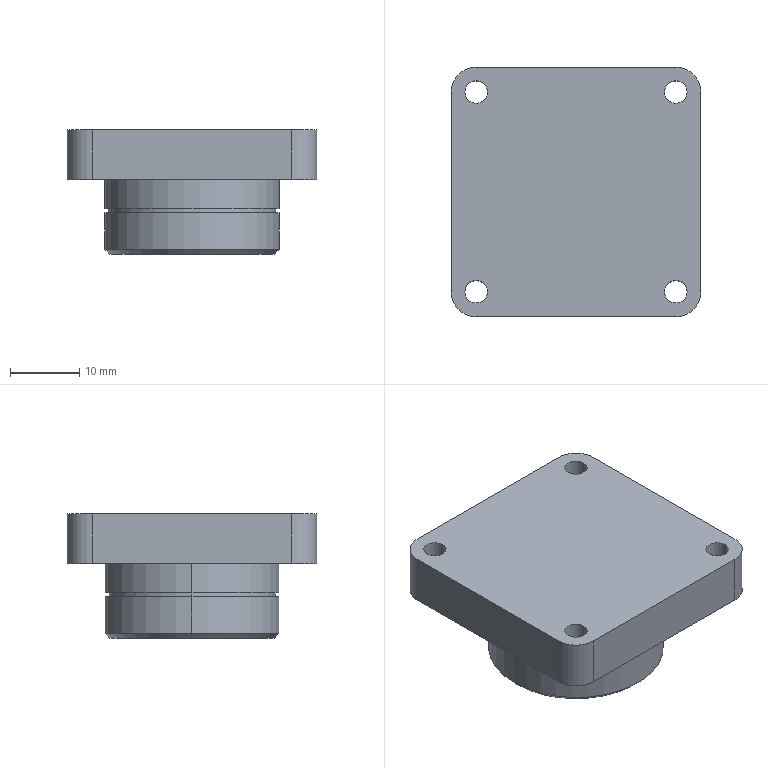Part | SolidWorks | features ICE 4, Chamfer 1, Extrusion 1, Fillet 1, RevCut 1 | 1 solid | 35 faces | box 36 x 36 x 18 mm | volume 11967 mm3 | cylinder 22 | plane 11 | cone 2 | commonest cylinder face diameters 3.24 x8 7.2 x4 25.2 x4 16.2 x2 24.12 x2 28.8 x2
STEP:
#1=CARTESIAN_POINT('',(8.1,0.,10.8));
#2=VERTEX_POINT('',#1);
#3=CARTESIAN_POINT('',(-8.1,0.,10.8));
#4=VERTEX_POINT('',#3);
#5=CARTESIAN_POINT('',(0.,0.,10.8));
#6=DIRECTION('',(0.,0.,-1.));
#7=DIRECTION('',(-1.,0.,0.));
#8=AXIS2_PLACEMENT_3D('',#5,#6,#7);
#9=CIRCLE('',#8,8.1);
#10=EDGE_CURVE('',#2,#4,#9,.T.);
#11=ORIENTED_EDGE('',*,*,#10,.F.);
#12=CARTESIAN_POINT('',(8.1,0.,0.));
#13=VERTEX_POINT('',#12);
#14=CARTESIAN_POINT('',(8.1,0.,10.8));
#15=DIRECTION('',(0.,0.,-1.));
#16=VECTOR('',#15,1000.);
#17=LINE('',#14,#16);
#18=EDGE_CURVE('',#2,#13,#17,.T.);
#19=ORIENTED_EDGE('',*,*,#18,.T.);
#20=CARTESIAN_POINT('',(-8.1,0.,0.));
#21=VERTEX_POINT('',#20);
#22=CARTESIAN_POINT('',(0.,0.,0.));
#23=DIRECTION('',(0.,0.,-1.));
#24=DIRECTION('',(-1.,0.,0.));
#25=AXIS2_PLACEMENT_3D('',#22,#23,#24);
#26=CIRCLE('',#25,8.1);
#27=EDGE_CURVE('',#13,#21,#26,.T.);
#28=ORIENTED_EDGE('',*,*,#27,.T.);
#29=CARTESIAN_POINT('',(-8.1,0.,10.8));
#30=DIRECTION('',(0.,0.,-1.));
#31=VECTOR('',#30,1000.);
#32=LINE('',#29,#31);
#33=EDGE_CURVE('',#4,#21,#32,.T.);
#34=ORIENTED_EDGE('',*,*,#33,.F.);
#35=EDGE_LOOP('',(#11,#19,#28,#34));
#36=FACE_OUTER_BOUND('',#35,.T.);
#37=CARTESIAN_POINT('',(0.,0.,10.8));
#38=DIRECTION('',(0.,0.,-1.));
#39=DIRECTION('',(-1.,0.,0.));
#40=AXIS2_PLACEMENT_3D('',#37,#38,#39);
#41=CYLINDRICAL_SURFACE('',#40,8.1);
#42=ADVANCED_FACE('',(#36),#41,.F.);
#43=CARTESIAN_POINT('',(12.78,14.4,18.));
#44=VERTEX_POINT('',#43);
#45=CARTESIAN_POINT('',(16.02,14.4,18.));
#46=VERTEX_POINT('',#45);
#47=CARTESIAN_POINT('',(14.4,14.4,18.));
#48=DIRECTION('',(0.,0.,1.));
#49=DIRECTION('',(-1.,0.,0.));
#50=AXIS2_PLACEMENT_3D('',#47,#48,#49);
#51=CIRCLE('',#50,1.62);
#52=EDGE_CURVE('',#44,#46,#51,.T.);
#53=ORIENTED_EDGE('',*,*,#52,.T.);
#54=CARTESIAN_POINT('',(16.02,14.4,10.8));
#55=VERTEX_POINT('',#54);
#56=CARTESIAN_POINT('',(16.02,14.4,22.582));
#57=DIRECTION('',(0.,0.,-1.));
#58=VECTOR('',#57,1000.);
#59=LINE('',#56,#58);
#60=EDGE_CURVE('',#46,#55,#59,.T.);
#61=ORIENTED_EDGE('',*,*,#60,.T.);
#62=CARTESIAN_POINT('',(12.78,14.4,10.8));
#63=VERTEX_POINT('',#62);
#64=CARTESIAN_POINT('',(14.4,14.4,10.8));
#65=DIRECTION('',(0.,0.,-1.));
#66=DIRECTION('',(-1.,0.,0.));
#67=AXIS2_PLACEMENT_3D('',#64,#65,#66);
#68=CIRCLE('',#67,1.62);
#69=EDGE_CURVE('',#55,#63,#68,.T.);
#70=ORIENTED_EDGE('',*,*,#69,.T.);
#71=CARTESIAN_POINT('',(12.78,14.4,22.582));
#72=DIRECTION('',(0.,0.,-1.));
#73=VECTOR('',#72,1000.);
#74=LINE('',#71,#73);
#75=EDGE_CURVE('',#44,#63,#74,.T.);
#76=ORIENTED_EDGE('',*,*,#75,.F.);
#77=EDGE_LOOP('',(#53,#61,#70,#76));
#78=FACE_OUTER_BOUND('',#77,.T.);
#79=CARTESIAN_POINT('',(14.4,14.4,22.582));
#80=DIRECTION('',(0.,0.,-1.));
#81=DIRECTION('',(-1.,0.,0.));
#82=AXIS2_PLACEMENT_3D('',#79,#80,#81);
#83=CYLINDRICAL_SURFACE('',#82,1.62);
#84=ADVANCED_FACE('',(#78),#83,.F.);
#85=CARTESIAN_POINT('',(12.78,-14.4,18.));
#86=VERTEX_POINT('',#85);
#87=CARTESIAN_POINT('',(16.02,-14.4,18.));
#88=VERTEX_POINT('',#87);
#89=CARTESIAN_POINT('',(14.4,-14.4,18.));
#90=DIRECTION('',(0.,0.,1.));
#91=DIRECTION('',(-1.,0.,0.));
#92=AXIS2_PLACEMENT_3D('',#89,#90,#91);
#93=CIRCLE('',#92,1.62);
#94=EDGE_CURVE('',#86,#88,#93,.T.);
#95=ORIENTED_EDGE('',*,*,#94,.T.);
#96=CARTESIAN_POINT('',(16.02,-14.4,10.8));
#97=VERTEX_POINT('',#96);
#98=CARTESIAN_POINT('',(16.02,-14.4,22.582));
#99=DIRECTION('',(0.,0.,-1.));
#100=VECTOR('',#99,1000.);
#101=LINE('',#98,#100);
#102=EDGE_CURVE('',#88,#97,#101,.T.);
#103=ORIENTED_EDGE('',*,*,#102,.T.);
#104=CARTESIAN_POINT('',(12.78,-14.4,10.8));
#105=VERTEX_POINT('',#104);
#106=CARTESIAN_POINT('',(14.4,-14.4,10.8));
#107=DIRECTION('',(0.,0.,-1.));
#108=DIRECTION('',(-1.,0.,0.));
#109=AXIS2_PLACEMENT_3D('',#106,#107,#108);
#110=CIRCLE('',#109,1.62);
#111=EDGE_CURVE('',#97,#105,#110,.T.);
#112=ORIENTED_EDGE('',*,*,#111,.T.);
#113=CARTESIAN_POINT('',(12.78,-14.4,22.582));
#114=DIRECTION('',(0.,0.,-1.));
#115=VECTOR('',#114,1000.);
#116=LINE('',#113,#115);
#117=EDGE_CURVE('',#86,#105,#116,.T.);
#118=ORIENTED_EDGE('',*,*,#117,.F.);
#119=EDGE_LOOP('',(#95,#103,#112,#118));
#120=FACE_OUTER_BOUND('',#119,.T.);
#121=CARTESIAN_POINT('',(14.4,-14.4,22.582));
#122=DIRECTION('',(0.,0.,-1.));
#123=DIRECTION('',(-1.,0.,0.));
#124=AXIS2_PLACEMENT_3D('',#121,#122,#123);
#125=CYLINDRICAL_SURFACE('',#124,1.62);
#126=ADVANCED_FACE('',(#120),#125,.F.);
#127=CARTESIAN_POINT('',(-16.02,-14.4,18.));
#128=VERTEX_POINT('',#127);
#129=CARTESIAN_POINT('',(-12.78,-14.4,18.));
#130=VERTEX_POINT('',#129);
#131=CARTESIAN_POINT('',(-14.4,-14.4,18.));
#132=DIRECTION('',(0.,0.,1.));
#133=DIRECTION('',(-1.,0.,0.));
#134=AXIS2_PLACEMENT_3D('',#131,#132,#133);
#135=CIRCLE('',#134,1.62);
#136=EDGE_CURVE('',#128,#130,#135,.T.);
#137=ORIENTED_EDGE('',*,*,#136,.T.);
#138=CARTESIAN_POINT('',(-12.78,-14.4,10.8));
#139=VERTEX_POINT('',#138);
#140=CARTESIAN_POINT('',(-12.78,-14.4,22.582));
#141=DIRECTION('',(0.,0.,-1.));
#142=VECTOR('',#141,1000.);
#143=LINE('',#140,#142);
#144=EDGE_CURVE('',#130,#139,#143,.T.);
#145=ORIENTED_EDGE('',*,*,#144,.T.);
#146=CARTESIAN_POINT('',(-16.02,-14.4,10.8));
#147=VERTEX_POINT('',#146);
#148=CARTESIAN_POINT('',(-14.4,-14.4,10.8));
#149=DIRECTION('',(0.,0.,-1.));
#150=DIRECTION('',(-1.,0.,0.));
#151=AXIS2_PLACEMENT_3D('',#148,#149,#150);
#152=CIRCLE('',#151,1.62);
#153=EDGE_CURVE('',#139,#147,#152,.T.);
#154=ORIENTED_EDGE('',*,*,#153,.T.);
#155=CARTESIAN_POINT('',(-16.02,-14.4,22.582));
#156=DIRECTION('',(0.,0.,-1.));
#157=VECTOR('',#156,1000.);
#158=LINE('',#155,#157);
#159=EDGE_CURVE('',#128,#147,#158,.T.);
#160=ORIENTED_EDGE('',*,*,#159,.F.);
#161=EDGE_LOOP('',(#137,#145,#154,#160));
#162=FACE_OUTER_BOUND('',#161,.T.);
#163=CARTESIAN_POINT('',(-14.4,-14.4,22.582));
#164=DIRECTION('',(0.,0.,-1.));
#165=DIRECTION('',(-1.,0.,0.));
#166=AXIS2_PLACEMENT_3D('',#163,#164,#165);
#167=CYLINDRICAL_SURFACE('',#166,1.62);
#168=ADVANCED_FACE('',(#162),#167,.F.);
#169=CARTESIAN_POINT('',(-16.02,14.4,18.));
#170=VERTEX_POINT('',#169);
#171=CARTESIAN_POINT('',(-12.78,14.4,18.));
#172=VERTEX_POINT('',#171);
#173=CARTESIAN_POINT('',(-14.4,14.4,18.));
#174=DIRECTION('',(0.,0.,1.));
#175=DIRECTION('',(-1.,0.,0.));
#176=AXIS2_PLACEMENT_3D('',#173,#174,#175);
#177=CIRCLE('',#176,1.62);
#178=EDGE_CURVE('',#170,#172,#177,.T.);
#179=ORIENTED_EDGE('',*,*,#178,.T.);
#180=CARTESIAN_POINT('',(-12.78,14.4,10.8));
#181=VERTEX_POINT('',#180);
#182=CARTESIAN_POINT('',(-12.78,14.4,22.582));
#183=DIRECTION('',(0.,0.,-1.));
#184=VECTOR('',#183,1000.);
#185=LINE('',#182,#184);
#186=EDGE_CURVE('',#172,#181,#185,.T.);
#187=ORIENTED_EDGE('',*,*,#186,.T.);
#188=CARTESIAN_POINT('',(-16.02,14.4,10.8));
#189=VERTEX_POINT('',#188);
#190=CARTESIAN_POINT('',(-14.4,14.4,10.8));
#191=DIRECTION('',(0.,0.,-1.));
#192=DIRECTION('',(-1.,0.,0.));
#193=AXIS2_PLACEMENT_3D('',#190,#191,#192);
#194=CIRCLE('',#193,1.62);
#195=EDGE_CURVE('',#181,#189,#194,.T.);
#196=ORIENTED_EDGE('',*,*,#195,.T.);
#197=CARTESIAN_POINT('',(-16.02,14.4,22.582));
#198=DIRECTION('',(0.,0.,-1.));
#199=VECTOR('',#198,1000.);
#200=LINE('',#197,#199);
#201=EDGE_CURVE('',#170,#189,#200,.T.);
#202=ORIENTED_EDGE('',*,*,#201,.F.);
#203=EDGE_LOOP('',(#179,#187,#196,#202));
#204=FACE_OUTER_BOUND('',#203,.T.);
#205=CARTESIAN_POINT('',(-14.4,14.4,22.582));
#206=DIRECTION('',(0.,0.,-1.));
#207=DIRECTION('',(-1.,0.,0.));
#208=AXIS2_PLACEMENT_3D('',#205,#206,#207);
#209=CYLINDRICAL_SURFACE('',#208,1.62);
#210=ADVANCED_FACE('',(#204),#209,.F.);
#211=CARTESIAN_POINT('',(12.6,0.,6.03));
#212=VERTEX_POINT('',#211);
#213=CARTESIAN_POINT('',(-12.6,0.,6.03));
#214=VERTEX_POINT('',#213);
#215=CARTESIAN_POINT('',(0.,0.,6.03));
#216=DIRECTION('',(0.,0.,1.));
#217=DIRECTION('',(1.,0.,0.));
#218=AXIS2_PLACEMENT_3D('',#215,#216,#217);
#219=CIRCLE('',#218,12.6);
#220=EDGE_CURVE('',#212,#214,#219,.T.);
#221=ORIENTED_EDGE('',*,*,#220,.F.);
#222=CARTESIAN_POINT('',(12.6,0.,0.72));
#223=VERTEX_POINT('',#222);
#224=CARTESIAN_POINT('',(12.6,0.,10.8));
#225=DIRECTION('',(0.,0.,-1.));
#226=VECTOR('',#225,1000.);
#227=LINE('',#224,#226);
#228=EDGE_CURVE('',#212,#223,#227,.T.);
#229=ORIENTED_EDGE('',*,*,#228,.T.);
#230=CARTESIAN_POINT('',(-12.6,0.,0.72));
#231=VERTEX_POINT('',#230);
#232=CARTESIAN_POINT('',(0.,0.,0.72));
#233=DIRECTION('',(0.,0.,1.));
#234=DIRECTION('',(1.,0.,0.));
#235=AXIS2_PLACEMENT_3D('',#232,#233,#234);
#236=CIRCLE('',#235,12.6);
#237=EDGE_CURVE('',#223,#231,#236,.T.);
#238=ORIENTED_EDGE('',*,*,#237,.T.);
#239=CARTESIAN_POINT('',(-12.6,0.,10.8));
#240=DIRECTION('',(0.,0.,-1.));
#241=VECTOR('',#240,1000.);
#242=LINE('',#239,#241);
#243=EDGE_CURVE('',#214,#231,#242,.T.);
#244=ORIENTED_EDGE('',*,*,#243,.F.);
#245=EDGE_LOOP('',(#221,#229,#238,#244));
#246=FACE_OUTER_BOUND('',#245,.T.);
#247=CARTESIAN_POINT('',(0.,0.,10.8));
#248=DIRECTION('',(0.,0.,-1.));
#249=DIRECTION('',(-1.,0.,0.));
#250=AXIS2_PLACEMENT_3D('',#247,#248,#249);
#251=CYLINDRICAL_SURFACE('',#250,12.6);
#252=ADVANCED_FACE('',(#246),#251,.T.);
#253=CARTESIAN_POINT('',(-11.88,0.,0.));
#254=VERTEX_POINT('',#253);
#255=CARTESIAN_POINT('',(11.88,0.,0.));
#256=VERTEX_POINT('',#255);
#257=CARTESIAN_POINT('',(0.,0.,0.));
#258=DIRECTION('',(0.,0.,-1.));
#259=DIRECTION('',(1.,0.,0.));
#260=AXIS2_PLACEMENT_3D('',#257,#258,#259);
#261=CIRCLE('',#260,11.88);
#262=EDGE_CURVE('',#254,#256,#261,.T.);
#263=ORIENTED_EDGE('',*,*,#262,.F.);
#264=CARTESIAN_POINT('',(-12.6,0.,0.72));
#265=DIRECTION('',(-0.7071,0.,0.7071));
#266=VECTOR('',#265,1000.);
#267=LINE('',#264,#266);
#268=EDGE_CURVE('',#254,#231,#267,.T.);
#269=ORIENTED_EDGE('',*,*,#268,.T.);
#270=ORIENTED_EDGE('',*,*,#237,.F.);
#271=CARTESIAN_POINT('',(12.6,0.,0.72));
#272=DIRECTION('',(0.7071,0.,0.7071));
#273=VECTOR('',#272,1000.);
#274=LINE('',#271,#273);
#275=EDGE_CURVE('',#256,#223,#274,.T.);
#276=ORIENTED_EDGE('',*,*,#275,.F.);
#277=EDGE_LOOP('',(#263,#269,#270,#276));
#278=FACE_OUTER_BOUND('',#277,.T.);
#279=CARTESIAN_POINT('',(0.,0.,0.72));
#280=DIRECTION('',(0.,0.,1.));
#281=DIRECTION('',(1.,0.,0.));
#282=AXIS2_PLACEMENT_3D('',#279,#280,#281);
#283=CONICAL_SURFACE('',#282,12.6,0.7854);
#284=ADVANCED_FACE('',(#278),#283,.T.);
#285=CARTESIAN_POINT('',(-12.06,0.,6.57));
#286=VERTEX_POINT('',#285);
#287=CARTESIAN_POINT('',(12.06,0.,6.57));
#288=VERTEX_POINT('',#287);
#289=CARTESIAN_POINT('',(0.,0.,6.57));
#290=DIRECTION('',(0.,0.,-1.));
#291=DIRECTION('',(-1.,0.,0.));
#292=AXIS2_PLACEMENT_3D('',#289,#290,#291);
#293=CIRCLE('',#292,12.06);
#294=EDGE_CURVE('',#286,#288,#293,.T.);
#295=ORIENTED_EDGE('',*,*,#294,.T.);
#296=CARTESIAN_POINT('',(12.06,0.,6.03));
#297=VERTEX_POINT('',#296);
#298=CARTESIAN_POINT('',(12.06,0.,-2.747));
#299=DIRECTION('',(0.,0.,-1.));
#300=VECTOR('',#299,1000.);
#301=LINE('',#298,#300);
#302=EDGE_CURVE('',#288,#297,#301,.T.);
#303=ORIENTED_EDGE('',*,*,#302,.T.);
#304=CARTESIAN_POINT('',(-12.06,0.,6.03));
#305=VERTEX_POINT('',#304);
#306=CARTESIAN_POINT('',(0.,0.,6.03));
#307=DIRECTION('',(0.,0.,-1.));
#308=DIRECTION('',(-1.,0.,0.));
#309=AXIS2_PLACEMENT_3D('',#306,#307,#308);
#310=CIRCLE('',#309,12.06);
#311=EDGE_CURVE('',#305,#297,#310,.T.);
#312=ORIENTED_EDGE('',*,*,#311,.F.);
#313=CARTESIAN_POINT('',(-12.06,0.,-2.747));
#314=DIRECTION('',(0.,0.,-1.));
#315=VECTOR('',#314,1000.);
#316=LINE('',#313,#315);
#317=EDGE_CURVE('',#286,#305,#316,.T.);
#318=ORIENTED_EDGE('',*,*,#317,.F.);
#319=EDGE_LOOP('',(#295,#303,#312,#318));
#320=FACE_OUTER_BOUND('',#319,.T.);
#321=CARTESIAN_POINT('',(0.,0.,-2.747));
#322=DIRECTION('',(0.,0.,-1.));
#323=DIRECTION('',(-1.,0.,0.));
#324=AXIS2_PLACEMENT_3D('',#321,#322,#323);
#325=CYLINDRICAL_SURFACE('',#324,12.06);
#326=ADVANCED_FACE('',(#320),#325,.T.);
#327=CARTESIAN_POINT('',(14.4,0.,11.88));
#328=VERTEX_POINT('',#327);
#329=CARTESIAN_POINT('',(-14.4,0.,11.88));
#330=VERTEX_POINT('',#329);
#331=CARTESIAN_POINT('',(0.,0.,11.88));
#332=DIRECTION('',(0.,0.,-1.));
#333=DIRECTION('',(-1.,0.,0.));
#334=AXIS2_PLACEMENT_3D('',#331,#332,#333);
#335=CIRCLE('',#334,14.4);
#336=EDGE_CURVE('',#328,#330,#335,.T.);
#337=ORIENTED_EDGE('',*,*,#336,.F.);
#338=CARTESIAN_POINT('',(14.4,0.,10.8));
#339=VERTEX_POINT('',#338);
#340=CARTESIAN_POINT('',(14.4,0.,11.88));
#341=DIRECTION('',(0.,0.,-1.));
#342=VECTOR('',#341,1000.);
#343=LINE('',#340,#342);
#344=EDGE_CURVE('',#328,#339,#343,.T.);
#345=ORIENTED_EDGE('',*,*,#344,.T.);
#346=CARTESIAN_POINT('',(-14.4,0.,10.8));
#347=VERTEX_POINT('',#346);
#348=CARTESIAN_POINT('',(0.,0.,10.8));
#349=DIRECTION('',(0.,0.,-1.));
#350=DIRECTION('',(-1.,0.,0.));
#351=AXIS2_PLACEMENT_3D('',#348,#349,#350);
#352=CIRCLE('',#351,14.4);
#353=EDGE_CURVE('',#339,#347,#352,.T.);
#354=ORIENTED_EDGE('',*,*,#353,.T.);
#355=CARTESIAN_POINT('',(-14.4,0.,11.88));
#356=DIRECTION('',(0.,0.,-1.));
#357=VECTOR('',#356,1000.);
#358=LINE('',#355,#357);
#359=EDGE_CURVE('',#330,#347,#358,.T.);
#360=ORIENTED_EDGE('',*,*,#359,.F.);
#361=EDGE_LOOP('',(#337,#345,#354,#360));
#362=FACE_OUTER_BOUND('',#361,.T.);
#363=CARTESIAN_POINT('',(0.,0.,11.88));
#364=DIRECTION('',(0.,0.,-1.));
#365=DIRECTION('',(-1.,0.,0.));
#366=AXIS2_PLACEMENT_3D('',#363,#364,#365);
#367=CYLINDRICAL_SURFACE('',#366,14.4);
#368=ADVANCED_FACE('',(#362),#367,.F.);
#369=CARTESIAN_POINT('',(-12.6,0.,11.88));
#370=VERTEX_POINT('',#369);
#371=CARTESIAN_POINT('',(12.6,0.,11.88));
#372=VERTEX_POINT('',#371);
#373=CARTESIAN_POINT('',(0.,0.,11.88));
#374=DIRECTION('',(0.,0.,-1.));
#375=DIRECTION('',(-1.,0.,0.));
#376=AXIS2_PLACEMENT_3D('',#373,#374,#375);
#377=CIRCLE('',#376,12.6);
#378=EDGE_CURVE('',#370,#372,#377,.T.);
#379=ORIENTED_EDGE('',*,*,#378,.T.);
#380=CARTESIAN_POINT('',(12.6,0.,6.57));
#381=VERTEX_POINT('',#380);
#382=CARTESIAN_POINT('',(12.6,0.,10.8));
#383=DIRECTION('',(0.,0.,-1.));
#384=VECTOR('',#383,1000.);
#385=LINE('',#382,#384);
#386=EDGE_CURVE('',#372,#381,#385,.T.);
#387=ORIENTED_EDGE('',*,*,#386,.T.);
#388=CARTESIAN_POINT('',(-12.6,0.,6.57));
#389=VERTEX_POINT('',#388);
#390=CARTESIAN_POINT('',(0.,0.,6.57));
#391=DIRECTION('',(0.,0.,-1.));
#392=DIRECTION('',(-1.,0.,0.));
#393=AXIS2_PLACEMENT_3D('',#390,#391,#392);
#394=CIRCLE('',#393,12.6);
#395=EDGE_CURVE('',#389,#381,#394,.T.);
#396=ORIENTED_EDGE('',*,*,#395,.F.);
#397=CARTESIAN_POINT('',(-12.6,0.,10.8));
#398=DIRECTION('',(0.,0.,-1.));
#399=VECTOR('',#398,1000.);
#400=LINE('',#397,#399);
#401=EDGE_CURVE('',#370,#389,#400,.T.);
#402=ORIENTED_EDGE('',*,*,#401,.F.);
#403=EDGE_LOOP('',(#379,#387,#396,#402));
#404=FACE_OUTER_BOUND('',#403,.T.);
#405=CARTESIAN_POINT('',(0.,0.,10.8));
#406=DIRECTION('',(0.,0.,-1.));
#407=DIRECTION('',(-1.,0.,0.));
#408=AXIS2_PLACEMENT_3D('',#405,#406,#407);
#409=CYLINDRICAL_SURFACE('',#408,12.6);
#410=ADVANCED_FACE('',(#404),#409,.T.);
#411=ORIENTED_EDGE('',*,*,#386,.F.);
#412=CARTESIAN_POINT('',(0.,0.,11.88));
#413=DIRECTION('',(0.,0.,-1.));
#414=DIRECTION('',(-1.,0.,0.));
#415=AXIS2_PLACEMENT_3D('',#412,#413,#414);
#416=CIRCLE('',#415,12.6);
#417=EDGE_CURVE('',#372,#370,#416,.T.);
#418=ORIENTED_EDGE('',*,*,#417,.T.);
#419=ORIENTED_EDGE('',*,*,#401,.T.);
#420=CARTESIAN_POINT('',(0.,0.,6.57));
#421=DIRECTION('',(0.,0.,-1.));
#422=DIRECTION('',(-1.,0.,0.));
#423=AXIS2_PLACEMENT_3D('',#420,#421,#422);
#424=CIRCLE('',#423,12.6);
#425=EDGE_CURVE('',#381,#389,#424,.T.);
#426=ORIENTED_EDGE('',*,*,#425,.F.);
#427=EDGE_LOOP('',(#411,#418,#419,#426));
#428=FACE_OUTER_BOUND('',#427,.T.);
#429=CARTESIAN_POINT('',(0.,0.,10.8));
#430=DIRECTION('',(0.,0.,-1.));
#431=DIRECTION('',(-1.,0.,0.));
#432=AXIS2_PLACEMENT_3D('',#429,#430,#431);
#433=CYLINDRICAL_SURFACE('',#432,12.6);
#434=ADVANCED_FACE('',(#428),#433,.T.);
#435=CARTESIAN_POINT('',(18.,-14.4,18.));
#436=VERTEX_POINT('',#435);
#437=CARTESIAN_POINT('',(18.,14.4,18.));
#438=VERTEX_POINT('',#437);
#439=CARTESIAN_POINT('',(18.,-18.,18.));
#440=DIRECTION('',(0.,1.,0.));
#441=VECTOR('',#440,1000.);
#442=LINE('',#439,#441);
#443=EDGE_CURVE('',#436,#438,#442,.T.);
#444=ORIENTED_EDGE('',*,*,#443,.F.);
#445=CARTESIAN_POINT('',(18.,-14.4,10.8));
#446=VERTEX_POINT('',#445);
#447=CARTESIAN_POINT('',(18.,-14.4,18.));
#448=DIRECTION('',(0.,0.,-1.));
#449=VECTOR('',#448,1000.);
#450=LINE('',#447,#449);
#451=EDGE_CURVE('',#436,#446,#450,.T.);
#452=ORIENTED_EDGE('',*,*,#451,.T.);
#453=CARTESIAN_POINT('',(18.,14.4,10.8));
#454=VERTEX_POINT('',#453);
#455=CARTESIAN_POINT('',(18.,-18.,10.8));
#456=DIRECTION('',(0.,1.,0.));
#457=VECTOR('',#456,1000.);
#458=LINE('',#455,#457);
#459=EDGE_CURVE('',#446,#454,#458,.T.);
#460=ORIENTED_EDGE('',*,*,#459,.T.);
#461=CARTESIAN_POINT('',(18.,14.4,18.));
#462=DIRECTION('',(0.,0.,1.));
#463=VECTOR('',#462,1000.);
#464=LINE('',#461,#463);
#465=EDGE_CURVE('',#454,#438,#464,.T.);
#466=ORIENTED_EDGE('',*,*,#465,.T.);
#467=EDGE_LOOP('',(#444,#452,#460,#466));
#468=FACE_OUTER_BOUND('',#467,.T.);
#469=CARTESIAN_POINT('',(18.,-18.,18.));
#470=DIRECTION('',(-1.,0.,0.));
#471=DIRECTION('',(0.,0.,1.));
#472=AXIS2_PLACEMENT_3D('',#469,#470,#471);
#473=PLANE('',#472);
#474=ADVANCED_FACE('',(#468),#473,.F.);
#475=CARTESIAN_POINT('',(14.4,18.,10.8));
#476=VERTEX_POINT('',#475);
#477=CARTESIAN_POINT('',(-14.4,18.,10.8));
#478=VERTEX_POINT('',#477);
#479=CARTESIAN_POINT('',(-18.,18.,10.8));
#480=DIRECTION('',(-1.,0.,0.));
#481=VECTOR('',#480,1000.);
#482=LINE('',#479,#481);
#483=EDGE_CURVE('',#476,#478,#482,.T.);
#484=ORIENTED_EDGE('',*,*,#483,.T.);
#485=CARTESIAN_POINT('',(-14.4,18.,18.));
#486=VERTEX_POINT('',#485);
#487=CARTESIAN_POINT('',(-14.4,18.,18.));
#488=DIRECTION('',(0.,0.,1.));
#489=VECTOR('',#488,1000.);
#490=LINE('',#487,#489);
#491=EDGE_CURVE('',#478,#486,#490,.T.);
#492=ORIENTED_EDGE('',*,*,#491,.T.);
#493=CARTESIAN_POINT('',(14.4,18.,18.));
#494=VERTEX_POINT('',#493);
#495=CARTESIAN_POINT('',(-18.,18.,18.));
#496=DIRECTION('',(-1.,0.,0.));
#497=VECTOR('',#496,1000.);
#498=LINE('',#495,#497);
#499=EDGE_CURVE('',#494,#486,#498,.T.);
#500=ORIENTED_EDGE('',*,*,#499,.F.);
#501=CARTESIAN_POINT('',(14.4,18.,18.));
#502=DIRECTION('',(0.,0.,-1.));
#503=VECTOR('',#502,1000.);
#504=LINE('',#501,#503);
#505=EDGE_CURVE('',#494,#476,#504,.T.);
#506=ORIENTED_EDGE('',*,*,#505,.T.);
#507=EDGE_LOOP('',(#484,#492,#500,#506));
#508=FACE_OUTER_BOUND('',#507,.T.);
#509=CARTESIAN_POINT('',(-18.,18.,18.));
#510=DIRECTION('',(0.,-1.,0.));
#511=DIRECTION('',(0.,0.,-1.));
#512=AXIS2_PLACEMENT_3D('',#509,#510,#511);
#513=PLANE('',#512);
#514=ADVANCED_FACE('',(#508),#513,.F.);
#515=CARTESIAN_POINT('',(-18.,14.4,18.));
#516=VERTEX_POINT('',#515);
#517=CARTESIAN_POINT('',(-18.,-14.4,18.));
#518=VERTEX_POINT('',#517);
#519=CARTESIAN_POINT('',(-18.,-18.,18.));
#520=DIRECTION('',(0.,-1.,0.));
#521=VECTOR('',#520,1000.);
#522=LINE('',#519,#521);
#523=EDGE_CURVE('',#516,#518,#522,.T.);
#524=ORIENTED_EDGE('',*,*,#523,.F.);
#525=CARTESIAN_POINT('',(-18.,14.4,10.8));
#526=VERTEX_POINT('',#525);
#527=CARTESIAN_POINT('',(-18.,14.4,18.));
#528=DIRECTION('',(0.,0.,-1.));
#529=VECTOR('',#528,1000.);
#530=LINE('',#527,#529);
#531=EDGE_CURVE('',#516,#526,#530,.T.);
#532=ORIENTED_EDGE('',*,*,#531,.T.);
#533=CARTESIAN_POINT('',(-18.,-14.4,10.8));
#534=VERTEX_POINT('',#533);
#535=CARTESIAN_POINT('',(-18.,-18.,10.8));
#536=DIRECTION('',(0.,-1.,0.));
#537=VECTOR('',#536,1000.);
#538=LINE('',#535,#537);
#539=EDGE_CURVE('',#526,#534,#538,.T.);
#540=ORIENTED_EDGE('',*,*,#539,.T.);
#541=CARTESIAN_POINT('',(-18.,-14.4,18.));
#542=DIRECTION('',(0.,0.,1.));
#543=VECTOR('',#542,1000.);
#544=LINE('',#541,#543);
#545=EDGE_CURVE('',#534,#518,#544,.T.);
#546=ORIENTED_EDGE('',*,*,#545,.T.);
#547=EDGE_LOOP('',(#524,#532,#540,#546));
#548=FACE_OUTER_BOUND('',#547,.T.);
#549=CARTESIAN_POINT('',(-18.,-18.,18.));
#550=DIRECTION('',(1.,0.,0.));
#551=DIRECTION('',(0.,0.,-1.));
#552=AXIS2_PLACEMENT_3D('',#549,#550,#551);
#553=PLANE('',#552);
#554=ADVANCED_FACE('',(#548),#553,.F.);
#555=CARTESIAN_POINT('',(-14.4,-18.,18.));
#556=VERTEX_POINT('',#555);
#557=CARTESIAN_POINT('',(14.4,-18.,18.));
#558=VERTEX_POINT('',#557);
#559=CARTESIAN_POINT('',(-18.,-18.,18.));
#560=DIRECTION('',(1.,0.,0.));
#561=VECTOR('',#560,1000.);
#562=LINE('',#559,#561);
#563=EDGE_CURVE('',#556,#558,#562,.T.);
#564=ORIENTED_EDGE('',*,*,#563,.F.);
#565=CARTESIAN_POINT('',(-14.4,-18.,10.8));
#566=VERTEX_POINT('',#565);
#567=CARTESIAN_POINT('',(-14.4,-18.,18.));
#568=DIRECTION('',(0.,0.,-1.));
#569=VECTOR('',#568,1000.);
#570=LINE('',#567,#569);
#571=EDGE_CURVE('',#556,#566,#570,.T.);
#572=ORIENTED_EDGE('',*,*,#571,.T.);
#573=CARTESIAN_POINT('',(14.4,-18.,10.8));
#574=VERTEX_POINT('',#573);
#575=CARTESIAN_POINT('',(-18.,-18.,10.8));
#576=DIRECTION('',(1.,0.,0.));
#577=VECTOR('',#576,1000.);
#578=LINE('',#575,#577);
#579=EDGE_CURVE('',#566,#574,#578,.T.);
#580=ORIENTED_EDGE('',*,*,#579,.T.);
#581=CARTESIAN_POINT('',(14.4,-18.,18.));
#582=DIRECTION('',(0.,0.,1.));
#583=VECTOR('',#582,1000.);
#584=LINE('',#581,#583);
#585=EDGE_CURVE('',#574,#558,#584,.T.);
#586=ORIENTED_EDGE('',*,*,#585,.T.);
#587=EDGE_LOOP('',(#564,#572,#580,#586));
#588=FACE_OUTER_BOUND('',#587,.T.);
#589=CARTESIAN_POINT('',(-18.,-18.,18.));
#590=DIRECTION('',(0.,1.,0.));
#591=DIRECTION('',(0.,0.,1.));
#592=AXIS2_PLACEMENT_3D('',#589,#590,#591);
#593=PLANE('',#592);
#594=ADVANCED_FACE('',(#588),#593,.F.);
#595=ORIENTED_EDGE('',*,*,#52,.F.);
#596=CARTESIAN_POINT('',(14.4,14.4,18.));
#597=DIRECTION('',(0.,0.,1.));
#598=DIRECTION('',(-1.,0.,0.));
#599=AXIS2_PLACEMENT_3D('',#596,#597,#598);
#600=CIRCLE('',#599,1.62);
#601=EDGE_CURVE('',#46,#44,#600,.T.);
#602=ORIENTED_EDGE('',*,*,#601,.F.);
#603=EDGE_LOOP('',(#595,#602));
#604=FACE_BOUND('',#603,.T.);
#605=ORIENTED_EDGE('',*,*,#94,.F.);
#606=CARTESIAN_POINT('',(14.4,-14.4,18.));
#607=DIRECTION('',(0.,0.,1.));
#608=DIRECTION('',(-1.,0.,0.));
#609=AXIS2_PLACEMENT_3D('',#606,#607,#608);
#610=CIRCLE('',#609,1.62);
#611=EDGE_CURVE('',#88,#86,#610,.T.);
#612=ORIENTED_EDGE('',*,*,#611,.F.);
#613=EDGE_LOOP('',(#605,#612));
#614=FACE_BOUND('',#613,.T.);
#615=ORIENTED_EDGE('',*,*,#136,.F.);
#616=CARTESIAN_POINT('',(-14.4,-14.4,18.));
#617=DIRECTION('',(0.,0.,1.));
#618=DIRECTION('',(-1.,0.,0.));
#619=AXIS2_PLACEMENT_3D('',#616,#617,#618);
#620=CIRCLE('',#619,1.62);
#621=EDGE_CURVE('',#130,#128,#620,.T.);
#622=ORIENTED_EDGE('',*,*,#621,.F.);
#623=EDGE_LOOP('',(#615,#622));
#624=FACE_BOUND('',#623,.T.);
#625=ORIENTED_EDGE('',*,*,#178,.F.);
#626=CARTESIAN_POINT('',(-14.4,14.4,18.));
#627=DIRECTION('',(0.,0.,1.));
#628=DIRECTION('',(-1.,0.,0.));
#629=AXIS2_PLACEMENT_3D('',#626,#627,#628);
#630=CIRCLE('',#629,1.62);
#631=EDGE_CURVE('',#172,#170,#630,.T.);
#632=ORIENTED_EDGE('',*,*,#631,.F.);
#633=EDGE_LOOP('',(#625,#632));
#634=FACE_BOUND('',#633,.T.);
#635=ORIENTED_EDGE('',*,*,#499,.T.);
#636=CARTESIAN_POINT('',(-14.4,14.4,18.));
#637=DIRECTION('',(0.,0.,1.));
#638=DIRECTION('',(-1.,0.,0.));
#639=AXIS2_PLACEMENT_3D('',#636,#637,#638);
#640=CIRCLE('',#639,3.6);
#641=EDGE_CURVE('',#486,#516,#640,.T.);
#642=ORIENTED_EDGE('',*,*,#641,.T.);
#643=ORIENTED_EDGE('',*,*,#523,.T.);
#644=CARTESIAN_POINT('',(-14.4,-14.4,18.));
#645=DIRECTION('',(0.,0.,1.));
#646=DIRECTION('',(-1.,0.,0.));
#647=AXIS2_PLACEMENT_3D('',#644,#645,#646);
#648=CIRCLE('',#647,3.6);
#649=EDGE_CURVE('',#518,#556,#648,.T.);
#650=ORIENTED_EDGE('',*,*,#649,.T.);
#651=ORIENTED_EDGE('',*,*,#563,.T.);
#652=CARTESIAN_POINT('',(14.4,-14.4,18.));
#653=DIRECTION('',(0.,0.,1.));
#654=DIRECTION('',(-1.,0.,0.));
#655=AXIS2_PLACEMENT_3D('',#652,#653,#654);
#656=CIRCLE('',#655,3.6);
#657=EDGE_CURVE('',#558,#436,#656,.T.);
#658=ORIENTED_EDGE('',*,*,#657,.T.);
#659=ORIENTED_EDGE('',*,*,#443,.T.);
#660=CARTESIAN_POINT('',(14.4,14.4,18.));
#661=DIRECTION('',(0.,0.,1.));
#662=DIRECTION('',(-1.,0.,0.));
#663=AXIS2_PLACEMENT_3D('',#660,#661,#662);
#664=CIRCLE('',#663,3.6);
#665=EDGE_CURVE('',#438,#494,#664,.T.);
#666=ORIENTED_EDGE('',*,*,#665,.T.);
#667=EDGE_LOOP('',(#635,#642,#643,#650,#651,#658,#659,#666));
#668=FACE_OUTER_BOUND('',#667,.T.);
#669=CARTESIAN_POINT('',(0.,0.,18.));
#670=DIRECTION('',(0.,0.,-1.));
#671=DIRECTION('',(-1.,0.,0.));
#672=AXIS2_PLACEMENT_3D('',#669,#670,#671);
#673=PLANE('',#672);
#674=ADVANCED_FACE('',(#604,#614,#624,#634,#668),#673,.F.);
#675=CARTESIAN_POINT('',(14.4,14.4,10.8));
#676=DIRECTION('',(0.,0.,-1.));
#677=DIRECTION('',(-1.,0.,0.));
#678=AXIS2_PLACEMENT_3D('',#675,#676,#677);
#679=CIRCLE('',#678,1.62);
#680=EDGE_CURVE('',#63,#55,#679,.T.);
#681=ORIENTED_EDGE('',*,*,#680,.F.);
#682=ORIENTED_EDGE('',*,*,#69,.F.);
#683=EDGE_LOOP('',(#681,#682));
#684=FACE_BOUND('',#683,.T.);
#685=CARTESIAN_POINT('',(14.4,-14.4,10.8));
#686=DIRECTION('',(0.,0.,-1.));
#687=DIRECTION('',(-1.,0.,0.));
#688=AXIS2_PLACEMENT_3D('',#685,#686,#687);
#689=CIRCLE('',#688,1.62);
#690=EDGE_CURVE('',#105,#97,#689,.T.);
#691=ORIENTED_EDGE('',*,*,#690,.F.);
#692=ORIENTED_EDGE('',*,*,#111,.F.);
#693=EDGE_LOOP('',(#691,#692));
#694=FACE_BOUND('',#693,.T.);
#695=CARTESIAN_POINT('',(-14.4,-14.4,10.8));
#696=DIRECTION('',(0.,0.,-1.));
#697=DIRECTION('',(-1.,0.,0.));
#698=AXIS2_PLACEMENT_3D('',#695,#696,#697);
#699=CIRCLE('',#698,1.62);
#700=EDGE_CURVE('',#147,#139,#699,.T.);
#701=ORIENTED_EDGE('',*,*,#700,.F.);
#702=ORIENTED_EDGE('',*,*,#153,.F.);
#703=EDGE_LOOP('',(#701,#702));
#704=FACE_BOUND('',#703,.T.);
#705=CARTESIAN_POINT('',(-14.4,14.4,10.8));
#706=DIRECTION('',(0.,0.,-1.));
#707=DIRECTION('',(-1.,0.,0.));
#708=AXIS2_PLACEMENT_3D('',#705,#706,#707);
#709=CIRCLE('',#708,1.62);
#710=EDGE_CURVE('',#189,#181,#709,.T.);
#711=ORIENTED_EDGE('',*,*,#710,.F.);
#712=ORIENTED_EDGE('',*,*,#195,.F.);
#713=EDGE_LOOP('',(#711,#712));
#714=FACE_BOUND('',#713,.T.);
#715=CARTESIAN_POINT('',(0.,0.,10.8));
#716=DIRECTION('',(0.,0.,-1.));
#717=DIRECTION('',(-1.,0.,0.));
#718=AXIS2_PLACEMENT_3D('',#715,#716,#717);
#719=CIRCLE('',#718,14.4);
#720=EDGE_CURVE('',#347,#339,#719,.T.);
#721=ORIENTED_EDGE('',*,*,#720,.F.);
#722=ORIENTED_EDGE('',*,*,#353,.F.);
#723=EDGE_LOOP('',(#721,#722));
#724=FACE_BOUND('',#723,.T.);
#725=ORIENTED_EDGE('',*,*,#539,.F.);
#726=CARTESIAN_POINT('',(-14.4,14.4,10.8));
#727=DIRECTION('',(0.,0.,-1.));
#728=DIRECTION('',(-1.,0.,0.));
#729=AXIS2_PLACEMENT_3D('',#726,#727,#728);
#730=CIRCLE('',#729,3.6);
#731=EDGE_CURVE('',#526,#478,#730,.T.);
#732=ORIENTED_EDGE('',*,*,#731,.T.);
#733=ORIENTED_EDGE('',*,*,#483,.F.);
#734=CARTESIAN_POINT('',(14.4,14.4,10.8));
#735=DIRECTION('',(0.,0.,-1.));
#736=DIRECTION('',(-1.,0.,0.));
#737=AXIS2_PLACEMENT_3D('',#734,#735,#736);
#738=CIRCLE('',#737,3.6);
#739=EDGE_CURVE('',#476,#454,#738,.T.);
#740=ORIENTED_EDGE('',*,*,#739,.T.);
#741=ORIENTED_EDGE('',*,*,#459,.F.);
#742=CARTESIAN_POINT('',(14.4,-14.4,10.8));
#743=DIRECTION('',(0.,0.,-1.));
#744=DIRECTION('',(-1.,0.,0.));
#745=AXIS2_PLACEMENT_3D('',#742,#743,#744);
#746=CIRCLE('',#745,3.6);
#747=EDGE_CURVE('',#446,#574,#746,.T.);
#748=ORIENTED_EDGE('',*,*,#747,.T.);
#749=ORIENTED_EDGE('',*,*,#579,.F.);
#750=CARTESIAN_POINT('',(-14.4,-14.4,10.8));
#751=DIRECTION('',(0.,0.,-1.));
#752=DIRECTION('',(-1.,0.,0.));
#753=AXIS2_PLACEMENT_3D('',#750,#751,#752);
#754=CIRCLE('',#753,3.6);
#755=EDGE_CURVE('',#566,#534,#754,.T.);
#756=ORIENTED_EDGE('',*,*,#755,.T.);
#757=EDGE_LOOP('',(#725,#732,#733,#740,#741,#748,#749,#756));
#758=FACE_OUTER_BOUND('',#757,.T.);
#759=CARTESIAN_POINT('',(0.,0.,10.8));
#760=DIRECTION('',(0.,0.,-1.));
#761=DIRECTION('',(-1.,0.,0.));
#762=AXIS2_PLACEMENT_3D('',#759,#760,#761);
#763=PLANE('',#762);
#764=ADVANCED_FACE('',(#684,#694,#704,#714,#724,#758),#763,.T.);
#765=ORIENTED_EDGE('',*,*,#641,.F.);
#766=ORIENTED_EDGE('',*,*,#491,.F.);
#767=ORIENTED_EDGE('',*,*,#731,.F.);
#768=ORIENTED_EDGE('',*,*,#531,.F.);
#769=EDGE_LOOP('',(#765,#766,#767,#768));
#770=FACE_OUTER_BOUND('',#769,.T.);
#771=CARTESIAN_POINT('',(-14.4,14.4,18.));
#772=DIRECTION('',(0.,0.,-1.));
#773=DIRECTION('',(-1.,0.,0.));
#774=AXIS2_PLACEMENT_3D('',#771,#772,#773);
#775=CYLINDRICAL_SURFACE('',#774,3.6);
#776=ADVANCED_FACE('',(#770),#775,.T.);
#777=ORIENTED_EDGE('',*,*,#649,.F.);
#778=ORIENTED_EDGE('',*,*,#545,.F.);
#779=ORIENTED_EDGE('',*,*,#755,.F.);
#780=ORIENTED_EDGE('',*,*,#571,.F.);
#781=EDGE_LOOP('',(#777,#778,#779,#780));
#782=FACE_OUTER_BOUND('',#781,.T.);
#783=CARTESIAN_POINT('',(-14.4,-14.4,18.));
#784=DIRECTION('',(0.,0.,-1.));
#785=DIRECTION('',(-1.,0.,0.));
#786=AXIS2_PLACEMENT_3D('',#783,#784,#785);
#787=CYLINDRICAL_SURFACE('',#786,3.6);
#788=ADVANCED_FACE('',(#782),#787,.T.);
#789=ORIENTED_EDGE('',*,*,#657,.F.);
#790=ORIENTED_EDGE('',*,*,#585,.F.);
#791=ORIENTED_EDGE('',*,*,#747,.F.);
#792=ORIENTED_EDGE('',*,*,#451,.F.);
#793=EDGE_LOOP('',(#789,#790,#791,#792));
#794=FACE_OUTER_BOUND('',#793,.T.);
#795=CARTESIAN_POINT('',(14.4,-14.4,18.));
#796=DIRECTION('',(0.,0.,-1.));
#797=DIRECTION('',(-1.,0.,0.));
#798=AXIS2_PLACEMENT_3D('',#795,#796,#797);
#799=CYLINDRICAL_SURFACE('',#798,3.6);
#800=ADVANCED_FACE('',(#794),#799,.T.);
#801=ORIENTED_EDGE('',*,*,#665,.F.);
#802=ORIENTED_EDGE('',*,*,#465,.F.);
#803=ORIENTED_EDGE('',*,*,#739,.F.);
#804=ORIENTED_EDGE('',*,*,#505,.F.);
#805=EDGE_LOOP('',(#801,#802,#803,#804));
#806=FACE_OUTER_BOUND('',#805,.T.);
#807=CARTESIAN_POINT('',(14.4,14.4,18.));
#808=DIRECTION('',(0.,0.,-1.));
#809=DIRECTION('',(-1.,0.,0.));
#810=AXIS2_PLACEMENT_3D('',#807,#808,#809);
#811=CYLINDRICAL_SURFACE('',#810,3.6);
#812=ADVANCED_FACE('',(#806),#811,.T.);
#813=ORIENTED_EDGE('',*,*,#344,.F.);
#814=CARTESIAN_POINT('',(0.,0.,11.88));
#815=DIRECTION('',(0.,0.,-1.));
#816=DIRECTION('',(-1.,0.,0.));
#817=AXIS2_PLACEMENT_3D('',#814,#815,#816);
#818=CIRCLE('',#817,14.4);
#819=EDGE_CURVE('',#330,#328,#818,.T.);
#820=ORIENTED_EDGE('',*,*,#819,.F.);
#821=ORIENTED_EDGE('',*,*,#359,.T.);
#822=ORIENTED_EDGE('',*,*,#720,.T.);
#823=EDGE_LOOP('',(#813,#820,#821,#822));
#824=FACE_OUTER_BOUND('',#823,.T.);
#825=CARTESIAN_POINT('',(0.,0.,11.88));
#826=DIRECTION('',(0.,0.,-1.));
#827=DIRECTION('',(-1.,0.,0.));
#828=AXIS2_PLACEMENT_3D('',#825,#826,#827);
#829=CYLINDRICAL_SURFACE('',#828,14.4);
#830=ADVANCED_FACE('',(#824),#829,.F.);
#831=ORIENTED_EDGE('',*,*,#378,.F.);
#832=ORIENTED_EDGE('',*,*,#417,.F.);
#833=EDGE_LOOP('',(#831,#832));
#834=FACE_BOUND('',#833,.T.);
#835=ORIENTED_EDGE('',*,*,#819,.T.);
#836=ORIENTED_EDGE('',*,*,#336,.T.);
#837=EDGE_LOOP('',(#835,#836));
#838=FACE_OUTER_BOUND('',#837,.T.);
#839=CARTESIAN_POINT('',(0.,0.,11.88));
#840=DIRECTION('',(0.,0.,-1.));
#841=DIRECTION('',(-1.,0.,0.));
#842=AXIS2_PLACEMENT_3D('',#839,#840,#841);
#843=PLANE('',#842);
#844=ADVANCED_FACE('',(#834,#838),#843,.T.);
#845=ORIENTED_EDGE('',*,*,#294,.F.);
#846=CARTESIAN_POINT('',(0.,0.,6.57));
#847=DIRECTION('',(0.,0.,-1.));
#848=DIRECTION('',(-1.,0.,0.));
#849=AXIS2_PLACEMENT_3D('',#846,#847,#848);
#850=CIRCLE('',#849,12.06);
#851=EDGE_CURVE('',#288,#286,#850,.T.);
#852=ORIENTED_EDGE('',*,*,#851,.F.);
#853=EDGE_LOOP('',(#845,#852));
#854=FACE_BOUND('',#853,.T.);
#855=ORIENTED_EDGE('',*,*,#395,.T.);
#856=ORIENTED_EDGE('',*,*,#425,.T.);
#857=EDGE_LOOP('',(#855,#856));
#858=FACE_OUTER_BOUND('',#857,.T.);
#859=CARTESIAN_POINT('',(12.06,0.,6.57));
#860=DIRECTION('',(0.,0.,-1.));
#861=DIRECTION('',(-1.,0.,0.));
#862=AXIS2_PLACEMENT_3D('',#859,#860,#861);
#863=PLANE('',#862);
#864=ADVANCED_FACE('',(#854,#858),#863,.T.);
#865=ORIENTED_EDGE('',*,*,#311,.T.);
#866=CARTESIAN_POINT('',(0.,0.,6.03));
#867=DIRECTION('',(0.,0.,-1.));
#868=DIRECTION('',(-1.,0.,0.));
#869=AXIS2_PLACEMENT_3D('',#866,#867,#868);
#870=CIRCLE('',#869,12.06);
#871=EDGE_CURVE('',#297,#305,#870,.T.);
#872=ORIENTED_EDGE('',*,*,#871,.T.);
#873=EDGE_LOOP('',(#865,#872));
#874=FACE_BOUND('',#873,.T.);
#875=CARTESIAN_POINT('',(0.,0.,6.03));
#876=DIRECTION('',(0.,0.,1.));
#877=DIRECTION('',(1.,0.,0.));
#878=AXIS2_PLACEMENT_3D('',#875,#876,#877);
#879=CIRCLE('',#878,12.6);
#880=EDGE_CURVE('',#214,#212,#879,.T.);
#881=ORIENTED_EDGE('',*,*,#880,.T.);
#882=ORIENTED_EDGE('',*,*,#220,.T.);
#883=EDGE_LOOP('',(#881,#882));
#884=FACE_OUTER_BOUND('',#883,.T.);
#885=CARTESIAN_POINT('',(12.06,0.,6.03));
#886=DIRECTION('',(0.,0.,1.));
#887=DIRECTION('',(1.,0.,0.));
#888=AXIS2_PLACEMENT_3D('',#885,#886,#887);
#889=PLANE('',#888);
#890=ADVANCED_FACE('',(#874,#884),#889,.T.);
#891=ORIENTED_EDGE('',*,*,#302,.F.);
#892=ORIENTED_EDGE('',*,*,#851,.T.);
#893=ORIENTED_EDGE('',*,*,#317,.T.);
#894=ORIENTED_EDGE('',*,*,#871,.F.);
#895=EDGE_LOOP('',(#891,#892,#893,#894));
#896=FACE_OUTER_BOUND('',#895,.T.);
#897=CARTESIAN_POINT('',(0.,0.,-2.747));
#898=DIRECTION('',(0.,0.,-1.));
#899=DIRECTION('',(-1.,0.,0.));
#900=AXIS2_PLACEMENT_3D('',#897,#898,#899);
#901=CYLINDRICAL_SURFACE('',#900,12.06);
#902=ADVANCED_FACE('',(#896),#901,.T.);
#903=CARTESIAN_POINT('',(0.,0.,0.));
#904=DIRECTION('',(0.,0.,-1.));
#905=DIRECTION('',(-1.,0.,0.));
#906=AXIS2_PLACEMENT_3D('',#903,#904,#905);
#907=CIRCLE('',#906,8.1);
#908=EDGE_CURVE('',#21,#13,#907,.T.);
#909=ORIENTED_EDGE('',*,*,#908,.F.);
#910=ORIENTED_EDGE('',*,*,#27,.F.);
#911=EDGE_LOOP('',(#909,#910));
#912=FACE_BOUND('',#911,.T.);
#913=CARTESIAN_POINT('',(0.,0.,0.));
#914=DIRECTION('',(0.,0.,-1.));
#915=DIRECTION('',(1.,0.,0.));
#916=AXIS2_PLACEMENT_3D('',#913,#914,#915);
#917=CIRCLE('',#916,11.88);
#918=EDGE_CURVE('',#256,#254,#917,.T.);
#919=ORIENTED_EDGE('',*,*,#918,.T.);
#920=ORIENTED_EDGE('',*,*,#262,.T.);
#921=EDGE_LOOP('',(#919,#920));
#922=FACE_OUTER_BOUND('',#921,.T.);
#923=CARTESIAN_POINT('',(0.,0.,0.));
#924=DIRECTION('',(0.,0.,1.));
#925=DIRECTION('',(1.,0.,0.));
#926=AXIS2_PLACEMENT_3D('',#923,#924,#925);
#927=PLANE('',#926);
#928=ADVANCED_FACE('',(#912,#922),#927,.F.);
#929=ORIENTED_EDGE('',*,*,#268,.F.);
#930=ORIENTED_EDGE('',*,*,#918,.F.);
#931=ORIENTED_EDGE('',*,*,#275,.T.);
#932=CARTESIAN_POINT('',(0.,0.,0.72));
#933=DIRECTION('',(0.,0.,1.));
#934=DIRECTION('',(1.,0.,0.));
#935=AXIS2_PLACEMENT_3D('',#932,#933,#934);
#936=CIRCLE('',#935,12.6);
#937=EDGE_CURVE('',#231,#223,#936,.T.);
#938=ORIENTED_EDGE('',*,*,#937,.F.);
#939=EDGE_LOOP('',(#929,#930,#931,#938));
#940=FACE_OUTER_BOUND('',#939,.T.);
#941=CARTESIAN_POINT('',(0.,0.,0.72));
#942=DIRECTION('',(0.,0.,1.));
#943=DIRECTION('',(1.,0.,0.));
#944=AXIS2_PLACEMENT_3D('',#941,#942,#943);
#945=CONICAL_SURFACE('',#944,12.6,0.7854);
#946=ADVANCED_FACE('',(#940),#945,.T.);
#947=ORIENTED_EDGE('',*,*,#228,.F.);
#948=ORIENTED_EDGE('',*,*,#880,.F.);
#949=ORIENTED_EDGE('',*,*,#243,.T.);
#950=ORIENTED_EDGE('',*,*,#937,.T.);
#951=EDGE_LOOP('',(#947,#948,#949,#950));
#952=FACE_OUTER_BOUND('',#951,.T.);
#953=CARTESIAN_POINT('',(0.,0.,10.8));
#954=DIRECTION('',(0.,0.,-1.));
#955=DIRECTION('',(-1.,0.,0.));
#956=AXIS2_PLACEMENT_3D('',#953,#954,#955);
#957=CYLINDRICAL_SURFACE('',#956,12.6);
#958=ADVANCED_FACE('',(#952),#957,.T.);
#959=ORIENTED_EDGE('',*,*,#186,.F.);
#960=ORIENTED_EDGE('',*,*,#631,.T.);
#961=ORIENTED_EDGE('',*,*,#201,.T.);
#962=ORIENTED_EDGE('',*,*,#710,.T.);
#963=EDGE_LOOP('',(#959,#960,#961,#962));
#964=FACE_OUTER_BOUND('',#963,.T.);
#965=CARTESIAN_POINT('',(-14.4,14.4,22.582));
#966=DIRECTION('',(0.,0.,-1.));
#967=DIRECTION('',(-1.,0.,0.));
#968=AXIS2_PLACEMENT_3D('',#965,#966,#967);
#969=CYLINDRICAL_SURFACE('',#968,1.62);
#970=ADVANCED_FACE('',(#964),#969,.F.);
#971=ORIENTED_EDGE('',*,*,#144,.F.);
#972=ORIENTED_EDGE('',*,*,#621,.T.);
#973=ORIENTED_EDGE('',*,*,#159,.T.);
#974=ORIENTED_EDGE('',*,*,#700,.T.);
#975=EDGE_LOOP('',(#971,#972,#973,#974));
#976=FACE_OUTER_BOUND('',#975,.T.);
#977=CARTESIAN_POINT('',(-14.4,-14.4,22.582));
#978=DIRECTION('',(0.,0.,-1.));
#979=DIRECTION('',(-1.,0.,0.));
#980=AXIS2_PLACEMENT_3D('',#977,#978,#979);
#981=CYLINDRICAL_SURFACE('',#980,1.62);
#982=ADVANCED_FACE('',(#976),#981,.F.);
#983=ORIENTED_EDGE('',*,*,#102,.F.);
#984=ORIENTED_EDGE('',*,*,#611,.T.);
#985=ORIENTED_EDGE('',*,*,#117,.T.);
#986=ORIENTED_EDGE('',*,*,#690,.T.);
#987=EDGE_LOOP('',(#983,#984,#985,#986));
#988=FACE_OUTER_BOUND('',#987,.T.);
#989=CARTESIAN_POINT('',(14.4,-14.4,22.582));
#990=DIRECTION('',(0.,0.,-1.));
#991=DIRECTION('',(-1.,0.,0.));
#992=AXIS2_PLACEMENT_3D('',#989,#990,#991);
#993=CYLINDRICAL_SURFACE('',#992,1.62);
#994=ADVANCED_FACE('',(#988),#993,.F.);
#995=ORIENTED_EDGE('',*,*,#60,.F.);
#996=ORIENTED_EDGE('',*,*,#601,.T.);
#997=ORIENTED_EDGE('',*,*,#75,.T.);
#998=ORIENTED_EDGE('',*,*,#680,.T.);
#999=EDGE_LOOP('',(#995,#996,#997,#998));
#1000=FACE_OUTER_BOUND('',#999,.T.);
#1001=CARTESIAN_POINT('',(14.4,14.4,22.582));
#1002=DIRECTION('',(0.,0.,-1.));
#1003=DIRECTION('',(-1.,0.,0.));
#1004=AXIS2_PLACEMENT_3D('',#1001,#1002,#1003);
#1005=CYLINDRICAL_SURFACE('',#1004,1.62);
#1006=ADVANCED_FACE('',(#1000),#1005,.F.);
#1007=ORIENTED_EDGE('',*,*,#18,.F.);
#1008=CARTESIAN_POINT('',(0.,0.,10.8));
#1009=DIRECTION('',(0.,0.,-1.));
#1010=DIRECTION('',(-1.,0.,0.));
#1011=AXIS2_PLACEMENT_3D('',#1008,#1009,#1010);
#1012=CIRCLE('',#1011,8.1);
#1013=EDGE_CURVE('',#4,#2,#1012,.T.);
#1014=ORIENTED_EDGE('',*,*,#1013,.F.);
#1015=ORIENTED_EDGE('',*,*,#33,.T.);
#1016=ORIENTED_EDGE('',*,*,#908,.T.);
#1017=EDGE_LOOP('',(#1007,#1014,#1015,#1016));
#1018=FACE_OUTER_BOUND('',#1017,.T.);
#1019=CARTESIAN_POINT('',(0.,0.,10.8));
#1020=DIRECTION('',(0.,0.,-1.));
#1021=DIRECTION('',(-1.,0.,0.));
#1022=AXIS2_PLACEMENT_3D('',#1019,#1020,#1021);
#1023=CYLINDRICAL_SURFACE('',#1022,8.1);
#1024=ADVANCED_FACE('',(#1018),#1023,.F.);
#1025=ORIENTED_EDGE('',*,*,#1013,.T.);
#1026=ORIENTED_EDGE('',*,*,#10,.T.);
#1027=EDGE_LOOP('',(#1025,#1026));
#1028=FACE_OUTER_BOUND('',#1027,.T.);
#1029=CARTESIAN_POINT('',(0.,0.,10.8));
#1030=DIRECTION('',(0.,0.,-1.));
#1031=DIRECTION('',(-1.,0.,0.));
#1032=AXIS2_PLACEMENT_3D('',#1029,#1030,#1031);
#1033=PLANE('',#1032);
#1034=ADVANCED_FACE('',(#1028),#1033,.T.);
#1035=CLOSED_SHELL('',(#42,#84,#126,#168,#210,#252,#284,#326,#368,#410,#434,#474,#514,#554,#594,#674,#764,#776,#788,#800,#812,#830,#844,#864,#890,#902,#928,#946,#958,#970,#982,#994,#1006,#1024,#1034));
#1036=MANIFOLD_SOLID_BREP('',#1035);
#1037=CARTESIAN_POINT('',(0.,0.,0.));
#1038=DIRECTION('',(0.,0.,1.));
#1039=DIRECTION('',(1.,0.,0.));
#1040=AXIS2_PLACEMENT_3D('',#1037,#1038,#1039);
#1041=(LENGTH_UNIT()NAMED_UNIT(*)SI_UNIT(.MILLI.,.METRE.));
#1042=UNCERTAINTY_MEASURE_WITH_UNIT(LENGTH_MEASURE(0.00001),#1041,'','');
#1043=(NAMED_UNIT(*)PLANE_ANGLE_UNIT()SI_UNIT($,.RADIAN.));
#1044=(NAMED_UNIT(*)SI_UNIT($,.STERADIAN.)SOLID_ANGLE_UNIT());
#1045=(GEOMETRIC_REPRESENTATION_CONTEXT(3)GLOBAL_UNCERTAINTY_ASSIGNED_CONTEXT((#1042))GLOBAL_UNIT_ASSIGNED_CONTEXT((#1041,#1043,#1044))REPRESENTATION_CONTEXT('',''));
#1046=ADVANCED_BREP_SHAPE_REPRESENTATION('',(#1036,#1040),#1045);